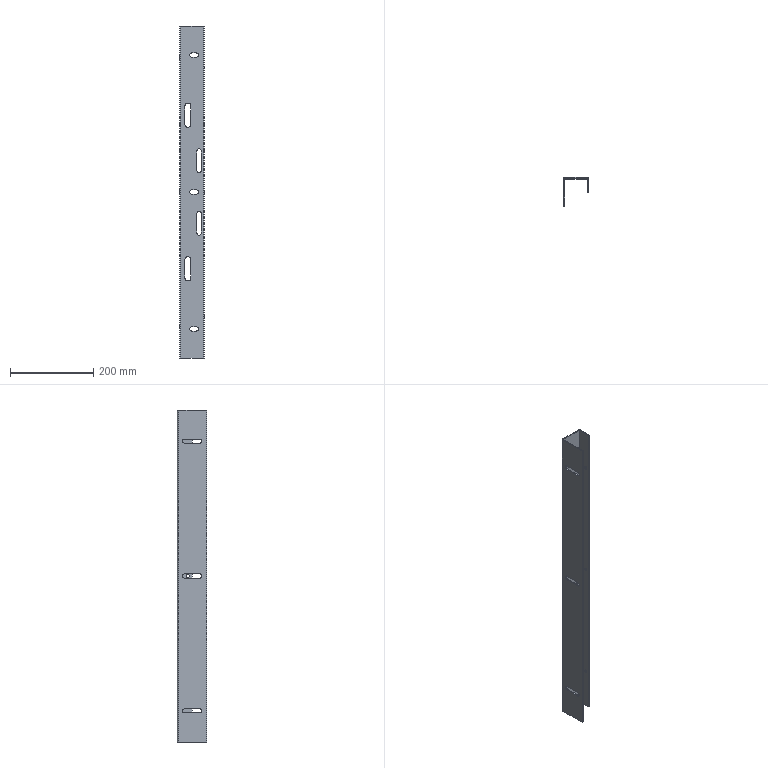Part | SolidWorks | features ICE 3, FlatPattern 1, SMBaseFlange 1, SheetMetal 1 | 1 solid | 71 faces | box 60 x 70 x 800 mm | volume 363963 mm3 | plane 38 | cylinder 33 | commonest cylinder face diameters 10 x19 7 x6 14 x4 0.4 x2 6.4 x2